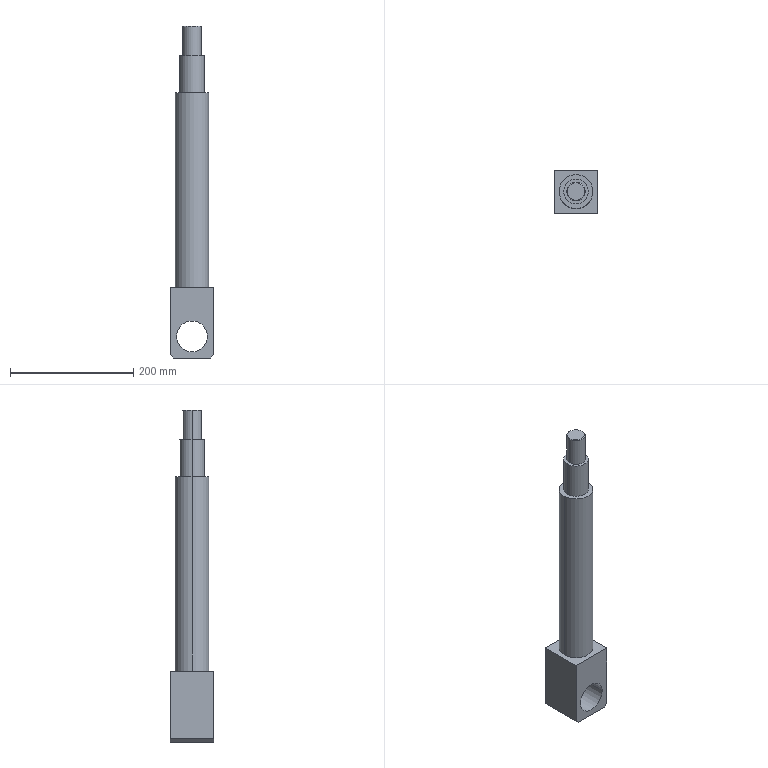Part | STEP file | LM-05-1239_default | 1 solid | 21 faces | box 70 x 70 x 538 mm | volume 1281973 mm3 | plane 11 | cylinder 8 | cone 2 | commonest cylinder face diameters 30 x2 40 x2 50 x2 55 x2
STEP:
#1=CARTESIAN_POINT('',(0.,0.,0.));
#2=DIRECTION('',(0.,0.,1.));
#3=DIRECTION('',(1.,0.,0.));
#4=AXIS2_PLACEMENT_3D('',#1,#2,#3);
#5=CARTESIAN_POINT('',(-25.,-35.,-80.));
#6=VERTEX_POINT('',#5);
#7=CARTESIAN_POINT('',(-25.,35.,-80.));
#8=VERTEX_POINT('',#7);
#9=CARTESIAN_POINT('',(-25.,-35.,-80.));
#10=DIRECTION('',(0.,1.,0.));
#11=VECTOR('',#10,1.);
#12=LINE('',#9,#11);
#13=CARTESIAN_POINT('',(0.,-35.,-80.));
#14=DIRECTION('',(0.,1.,0.));
#15=DIRECTION('',(-1.,0.,0.));
#16=AXIS2_PLACEMENT_3D('',#13,#14,#15);
#17=CYLINDRICAL_SURFACE('',#16,25.);
#18=CARTESIAN_POINT('',(6.283,0.));
#19=DIRECTION('',(0.,1.));
#20=VECTOR('',#19,1.);
#21=LINE('',#18,#20);
#22=(GEOMETRIC_REPRESENTATION_CONTEXT(2)PARAMETRIC_REPRESENTATION_CONTEXT()REPRESENTATION_CONTEXT('',''));
#23=DEFINITIONAL_REPRESENTATION('',(#21),#22);
#24=PCURVE('',#17,#23);
#25=CARTESIAN_POINT('',(0.,-35.,-80.));
#26=DIRECTION('',(0.,1.,0.));
#27=DIRECTION('',(-1.,0.,0.));
#28=AXIS2_PLACEMENT_3D('',#25,#26,#27);
#29=CYLINDRICAL_SURFACE('',#28,25.);
#30=CARTESIAN_POINT('',(0.,0.));
#31=DIRECTION('',(0.,1.));
#32=VECTOR('',#31,1.);
#33=LINE('',#30,#32);
#34=(GEOMETRIC_REPRESENTATION_CONTEXT(2)PARAMETRIC_REPRESENTATION_CONTEXT()REPRESENTATION_CONTEXT('',''));
#35=DEFINITIONAL_REPRESENTATION('',(#33),#34);
#36=PCURVE('',#29,#35);
#37=SURFACE_CURVE('',#12,(#24,#36),.PCURVE_S1.);
#38=EDGE_CURVE('',#6,#8,#37,.T.);
#39=ORIENTED_EDGE('',*,*,#38,.T.);
#40=CARTESIAN_POINT('',(25.,35.,-80.));
#41=VERTEX_POINT('',#40);
#42=CARTESIAN_POINT('',(0.,35.,-80.));
#43=DIRECTION('',(0.,1.,0.));
#44=DIRECTION('',(-1.,0.,0.));
#45=AXIS2_PLACEMENT_3D('',#42,#43,#44);
#46=CIRCLE('',#45,25.);
#47=CARTESIAN_POINT('',(0.,70.));
#48=DIRECTION('',(1.,0.));
#49=VECTOR('',#48,1.);
#50=LINE('',#47,#49);
#51=(GEOMETRIC_REPRESENTATION_CONTEXT(2)PARAMETRIC_REPRESENTATION_CONTEXT()REPRESENTATION_CONTEXT('',''));
#52=DEFINITIONAL_REPRESENTATION('',(#50),#51);
#53=PCURVE('',#17,#52);
#54=CARTESIAN_POINT('',(35.,35.,-115.));
#55=DIRECTION('',(0.,-1.,0.));
#56=DIRECTION('',(0.,0.,-1.));
#57=AXIS2_PLACEMENT_3D('',#54,#55,#56);
#58=PLANE('',#57);
#59=CARTESIAN_POINT('',(-35.,-60.));
#60=CARTESIAN_POINT('',(-78.301,-60.));
#61=CARTESIAN_POINT('',(-56.651,-22.5));
#62=CARTESIAN_POINT('',(-35.,15.));
#63=CARTESIAN_POINT('',(-13.349,-22.5));
#64=CARTESIAN_POINT('',(8.301,-60.));
#65=CARTESIAN_POINT('',(-35.,-60.));
#66=(BOUNDED_CURVE()B_SPLINE_CURVE(2,(#59,#60,#61,#62,#63,#64,#65),.UNSPECIFIED.,.T.,.F.)B_SPLINE_CURVE_WITH_KNOTS((1,2,2,2,2,1),(-2.094,0.,2.094,4.189,6.283,8.378),.UNSPECIFIED.)CURVE()GEOMETRIC_REPRESENTATION_ITEM()RATIONAL_B_SPLINE_CURVE((1.,0.5,1.,0.5,1.,0.5,1.))REPRESENTATION_ITEM(''));
#67=(GEOMETRIC_REPRESENTATION_CONTEXT(2)PARAMETRIC_REPRESENTATION_CONTEXT()REPRESENTATION_CONTEXT('',''));
#68=DEFINITIONAL_REPRESENTATION('',(#66),#67);
#69=PCURVE('',#58,#68);
#70=SURFACE_CURVE('',#46,(#53,#69),.PCURVE_S1.);
#71=EDGE_CURVE('',#41,#8,#70,.T.);
#72=ORIENTED_EDGE('',*,*,#71,.F.);
#73=CARTESIAN_POINT('',(25.,-35.,-80.));
#74=VERTEX_POINT('',#73);
#75=CARTESIAN_POINT('',(25.,-35.,-80.));
#76=DIRECTION('',(0.,1.,0.));
#77=VECTOR('',#76,1.);
#78=LINE('',#75,#77);
#79=CARTESIAN_POINT('',(3.142,0.));
#80=DIRECTION('',(0.,1.));
#81=VECTOR('',#80,1.);
#82=LINE('',#79,#81);
#83=(GEOMETRIC_REPRESENTATION_CONTEXT(2)PARAMETRIC_REPRESENTATION_CONTEXT()REPRESENTATION_CONTEXT('',''));
#84=DEFINITIONAL_REPRESENTATION('',(#82),#83);
#85=PCURVE('',#17,#84);
#86=CARTESIAN_POINT('',(3.142,0.));
#87=DIRECTION('',(0.,1.));
#88=VECTOR('',#87,1.);
#89=LINE('',#86,#88);
#90=(GEOMETRIC_REPRESENTATION_CONTEXT(2)PARAMETRIC_REPRESENTATION_CONTEXT()REPRESENTATION_CONTEXT('',''));
#91=DEFINITIONAL_REPRESENTATION('',(#89),#90);
#92=PCURVE('',#29,#91);
#93=SURFACE_CURVE('',#78,(#85,#92),.PCURVE_S1.);
#94=EDGE_CURVE('',#74,#41,#93,.T.);
#95=ORIENTED_EDGE('',*,*,#94,.F.);
#96=CARTESIAN_POINT('',(0.,-35.,-80.));
#97=DIRECTION('',(0.,1.,0.));
#98=DIRECTION('',(-1.,0.,0.));
#99=AXIS2_PLACEMENT_3D('',#96,#97,#98);
#100=CIRCLE('',#99,25.);
#101=CARTESIAN_POINT('',(0.,0.));
#102=DIRECTION('',(1.,0.));
#103=VECTOR('',#102,1.);
#104=LINE('',#101,#103);
#105=(GEOMETRIC_REPRESENTATION_CONTEXT(2)PARAMETRIC_REPRESENTATION_CONTEXT()REPRESENTATION_CONTEXT('',''));
#106=DEFINITIONAL_REPRESENTATION('',(#104),#105);
#107=PCURVE('',#17,#106);
#108=CARTESIAN_POINT('',(35.,-35.,-115.));
#109=DIRECTION('',(0.,1.,0.));
#110=DIRECTION('',(0.,0.,1.));
#111=AXIS2_PLACEMENT_3D('',#108,#109,#110);
#112=PLANE('',#111);
#113=CARTESIAN_POINT('',(35.,-35.));
#114=DIRECTION('',(0.,-1.));
#115=AXIS2_PLACEMENT_2D('',#113,#114);
#116=CIRCLE('',#115,25.);
#117=(GEOMETRIC_REPRESENTATION_CONTEXT(2)PARAMETRIC_REPRESENTATION_CONTEXT()REPRESENTATION_CONTEXT('',''));
#118=DEFINITIONAL_REPRESENTATION('',(#116),#117);
#119=PCURVE('',#112,#118);
#120=SURFACE_CURVE('',#100,(#107,#119),.PCURVE_S1.);
#121=EDGE_CURVE('',#74,#6,#120,.T.);
#122=ORIENTED_EDGE('',*,*,#121,.T.);
#123=EDGE_LOOP('',(#39,#72,#95,#122));
#124=FACE_BOUND('',#123,.F.);
#125=ADVANCED_FACE('',(#124),#17,.F.);
#126=CARTESIAN_POINT('',(20.,0.,315.));
#127=VERTEX_POINT('',#126);
#128=CARTESIAN_POINT('',(-20.,0.,315.));
#129=VERTEX_POINT('',#128);
#130=CARTESIAN_POINT('',(0.,0.,315.));
#131=DIRECTION('',(0.,0.,1.));
#132=DIRECTION('',(1.,0.,0.));
#133=AXIS2_PLACEMENT_3D('',#130,#131,#132);
#134=CIRCLE('',#133,20.);
#135=CARTESIAN_POINT('',(0.,0.,0.));
#136=DIRECTION('',(0.,0.,1.));
#137=DIRECTION('',(1.,0.,0.));
#138=AXIS2_PLACEMENT_3D('',#135,#136,#137);
#139=CYLINDRICAL_SURFACE('',#138,20.);
#140=CARTESIAN_POINT('',(0.,315.));
#141=DIRECTION('',(1.,0.));
#142=VECTOR('',#141,1.);
#143=LINE('',#140,#142);
#144=(GEOMETRIC_REPRESENTATION_CONTEXT(2)PARAMETRIC_REPRESENTATION_CONTEXT()REPRESENTATION_CONTEXT('',''));
#145=DEFINITIONAL_REPRESENTATION('',(#143),#144);
#146=PCURVE('',#139,#145);
#147=CARTESIAN_POINT('',(0.,20.,315.));
#148=DIRECTION('',(0.,0.,1.));
#149=DIRECTION('',(1.,0.,0.));
#150=AXIS2_PLACEMENT_3D('',#147,#148,#149);
#151=PLANE('',#150);
#152=CARTESIAN_POINT('',(0.,-20.));
#153=DIRECTION('',(1.,0.));
#154=AXIS2_PLACEMENT_2D('',#152,#153);
#155=CIRCLE('',#154,20.);
#156=(GEOMETRIC_REPRESENTATION_CONTEXT(2)PARAMETRIC_REPRESENTATION_CONTEXT()REPRESENTATION_CONTEXT('',''));
#157=DEFINITIONAL_REPRESENTATION('',(#155),#156);
#158=PCURVE('',#151,#157);
#159=SURFACE_CURVE('',#134,(#146,#158),.PCURVE_S1.);
#160=EDGE_CURVE('',#127,#129,#159,.T.);
#161=ORIENTED_EDGE('',*,*,#160,.T.);
#162=CARTESIAN_POINT('',(-20.,0.,375.));
#163=VERTEX_POINT('',#162);
#164=CARTESIAN_POINT('',(-20.,0.,0.));
#165=DIRECTION('',(0.,0.,1.));
#166=VECTOR('',#165,1.);
#167=LINE('',#164,#166);
#168=CARTESIAN_POINT('',(3.142,0.));
#169=DIRECTION('',(0.,1.));
#170=VECTOR('',#169,1.);
#171=LINE('',#168,#170);
#172=(GEOMETRIC_REPRESENTATION_CONTEXT(2)PARAMETRIC_REPRESENTATION_CONTEXT()REPRESENTATION_CONTEXT('',''));
#173=DEFINITIONAL_REPRESENTATION('',(#171),#172);
#174=PCURVE('',#139,#173);
#175=CARTESIAN_POINT('',(0.,0.,0.));
#176=DIRECTION('',(0.,0.,1.));
#177=DIRECTION('',(1.,0.,0.));
#178=AXIS2_PLACEMENT_3D('',#175,#176,#177);
#179=CYLINDRICAL_SURFACE('',#178,20.);
#180=CARTESIAN_POINT('',(3.142,0.));
#181=DIRECTION('',(0.,1.));
#182=VECTOR('',#181,1.);
#183=LINE('',#180,#182);
#184=(GEOMETRIC_REPRESENTATION_CONTEXT(2)PARAMETRIC_REPRESENTATION_CONTEXT()REPRESENTATION_CONTEXT('',''));
#185=DEFINITIONAL_REPRESENTATION('',(#183),#184);
#186=PCURVE('',#179,#185);
#187=SURFACE_CURVE('',#167,(#174,#186),.PCURVE_S1.);
#188=EDGE_CURVE('',#129,#163,#187,.T.);
#189=ORIENTED_EDGE('',*,*,#188,.T.);
#190=CARTESIAN_POINT('',(20.,0.,375.));
#191=VERTEX_POINT('',#190);
#192=CARTESIAN_POINT('',(0.,0.,375.));
#193=DIRECTION('',(0.,0.,1.));
#194=DIRECTION('',(1.,0.,0.));
#195=AXIS2_PLACEMENT_3D('',#192,#193,#194);
#196=CIRCLE('',#195,20.);
#197=CARTESIAN_POINT('',(0.,375.));
#198=DIRECTION('',(1.,0.));
#199=VECTOR('',#198,1.);
#200=LINE('',#197,#199);
#201=(GEOMETRIC_REPRESENTATION_CONTEXT(2)PARAMETRIC_REPRESENTATION_CONTEXT()REPRESENTATION_CONTEXT('',''));
#202=DEFINITIONAL_REPRESENTATION('',(#200),#201);
#203=PCURVE('',#139,#202);
#204=CARTESIAN_POINT('',(0.,0.,375.));
#205=DIRECTION('',(0.,0.,1.));
#206=DIRECTION('',(1.,0.,0.));
#207=AXIS2_PLACEMENT_3D('',#204,#205,#206);
#208=PLANE('',#207);
#209=CARTESIAN_POINT('',(0.,0.));
#210=DIRECTION('',(1.,0.));
#211=AXIS2_PLACEMENT_2D('',#209,#210);
#212=CIRCLE('',#211,20.);
#213=(GEOMETRIC_REPRESENTATION_CONTEXT(2)PARAMETRIC_REPRESENTATION_CONTEXT()REPRESENTATION_CONTEXT('',''));
#214=DEFINITIONAL_REPRESENTATION('',(#212),#213);
#215=PCURVE('',#208,#214);
#216=SURFACE_CURVE('',#196,(#203,#215),.PCURVE_S1.);
#217=EDGE_CURVE('',#191,#163,#216,.T.);
#218=ORIENTED_EDGE('',*,*,#217,.F.);
#219=CARTESIAN_POINT('',(20.,0.,0.));
#220=DIRECTION('',(0.,0.,1.));
#221=VECTOR('',#220,1.);
#222=LINE('',#219,#221);
#223=CARTESIAN_POINT('',(0.,0.));
#224=DIRECTION('',(0.,1.));
#225=VECTOR('',#224,1.);
#226=LINE('',#223,#225);
#227=(GEOMETRIC_REPRESENTATION_CONTEXT(2)PARAMETRIC_REPRESENTATION_CONTEXT()REPRESENTATION_CONTEXT('',''));
#228=DEFINITIONAL_REPRESENTATION('',(#226),#227);
#229=PCURVE('',#139,#228);
#230=CARTESIAN_POINT('',(6.283,0.));
#231=DIRECTION('',(0.,1.));
#232=VECTOR('',#231,1.);
#233=LINE('',#230,#232);
#234=(GEOMETRIC_REPRESENTATION_CONTEXT(2)PARAMETRIC_REPRESENTATION_CONTEXT()REPRESENTATION_CONTEXT('',''));
#235=DEFINITIONAL_REPRESENTATION('',(#233),#234);
#236=PCURVE('',#179,#235);
#237=SURFACE_CURVE('',#222,(#229,#236),.PCURVE_S1.);
#238=EDGE_CURVE('',#127,#191,#237,.T.);
#239=ORIENTED_EDGE('',*,*,#238,.F.);
#240=EDGE_LOOP('',(#161,#189,#218,#239));
#241=FACE_BOUND('',#240,.T.);
#242=ADVANCED_FACE('',(#241),#139,.T.);
#243=CARTESIAN_POINT('',(27.5,0.,0.));
#244=VERTEX_POINT('',#243);
#245=CARTESIAN_POINT('',(-27.5,0.,0.));
#246=VERTEX_POINT('',#245);
#247=CARTESIAN_POINT('',(0.,0.,0.));
#248=DIRECTION('',(0.,0.,1.));
#249=DIRECTION('',(1.,0.,0.));
#250=AXIS2_PLACEMENT_3D('',#247,#248,#249);
#251=CIRCLE('',#250,27.5);
#252=CARTESIAN_POINT('',(0.,0.,0.));
#253=DIRECTION('',(0.,0.,1.));
#254=DIRECTION('',(1.,0.,0.));
#255=AXIS2_PLACEMENT_3D('',#252,#253,#254);
#256=CYLINDRICAL_SURFACE('',#255,27.5);
#257=CARTESIAN_POINT('',(0.,0.));
#258=DIRECTION('',(1.,0.));
#259=VECTOR('',#258,1.);
#260=LINE('',#257,#259);
#261=(GEOMETRIC_REPRESENTATION_CONTEXT(2)PARAMETRIC_REPRESENTATION_CONTEXT()REPRESENTATION_CONTEXT('',''));
#262=DEFINITIONAL_REPRESENTATION('',(#260),#261);
#263=PCURVE('',#256,#262);
#264=CARTESIAN_POINT('',(0.,0.,0.));
#265=DIRECTION('',(0.,0.,-1.));
#266=DIRECTION('',(-1.,0.,0.));
#267=AXIS2_PLACEMENT_3D('',#264,#265,#266);
#268=PLANE('',#267);
#269=CARTESIAN_POINT('',(-27.5,0.));
#270=CARTESIAN_POINT('',(-27.5,47.631));
#271=CARTESIAN_POINT('',(13.75,23.816));
#272=CARTESIAN_POINT('',(55.,0.));
#273=CARTESIAN_POINT('',(13.75,-23.816));
#274=CARTESIAN_POINT('',(-27.5,-47.631));
#275=CARTESIAN_POINT('',(-27.5,0.));
#276=(BOUNDED_CURVE()B_SPLINE_CURVE(2,(#269,#270,#271,#272,#273,#274,#275),.UNSPECIFIED.,.T.,.F.)B_SPLINE_CURVE_WITH_KNOTS((1,2,2,2,2,1),(-2.094,0.,2.094,4.189,6.283,8.378),.UNSPECIFIED.)CURVE()GEOMETRIC_REPRESENTATION_ITEM()RATIONAL_B_SPLINE_CURVE((1.,0.5,1.,0.5,1.,0.5,1.))REPRESENTATION_ITEM(''));
#277=(GEOMETRIC_REPRESENTATION_CONTEXT(2)PARAMETRIC_REPRESENTATION_CONTEXT()REPRESENTATION_CONTEXT('',''));
#278=DEFINITIONAL_REPRESENTATION('',(#276),#277);
#279=PCURVE('',#268,#278);
#280=SURFACE_CURVE('',#251,(#263,#279),.PCURVE_S1.);
#281=EDGE_CURVE('',#244,#246,#280,.T.);
#282=ORIENTED_EDGE('',*,*,#281,.T.);
#283=CARTESIAN_POINT('',(-27.5,0.,315.));
#284=VERTEX_POINT('',#283);
#285=CARTESIAN_POINT('',(-27.5,0.,0.));
#286=DIRECTION('',(0.,0.,1.));
#287=VECTOR('',#286,1.);
#288=LINE('',#285,#287);
#289=CARTESIAN_POINT('',(3.142,0.));
#290=DIRECTION('',(0.,1.));
#291=VECTOR('',#290,1.);
#292=LINE('',#289,#291);
#293=(GEOMETRIC_REPRESENTATION_CONTEXT(2)PARAMETRIC_REPRESENTATION_CONTEXT()REPRESENTATION_CONTEXT('',''));
#294=DEFINITIONAL_REPRESENTATION('',(#292),#293);
#295=PCURVE('',#256,#294);
#296=CARTESIAN_POINT('',(0.,0.,0.));
#297=DIRECTION('',(0.,0.,1.));
#298=DIRECTION('',(1.,0.,0.));
#299=AXIS2_PLACEMENT_3D('',#296,#297,#298);
#300=CYLINDRICAL_SURFACE('',#299,27.5);
#301=CARTESIAN_POINT('',(3.142,0.));
#302=DIRECTION('',(0.,1.));
#303=VECTOR('',#302,1.);
#304=LINE('',#301,#303);
#305=(GEOMETRIC_REPRESENTATION_CONTEXT(2)PARAMETRIC_REPRESENTATION_CONTEXT()REPRESENTATION_CONTEXT('',''));
#306=DEFINITIONAL_REPRESENTATION('',(#304),#305);
#307=PCURVE('',#300,#306);
#308=SURFACE_CURVE('',#288,(#295,#307),.PCURVE_S1.);
#309=EDGE_CURVE('',#246,#284,#308,.T.);
#310=ORIENTED_EDGE('',*,*,#309,.T.);
#311=CARTESIAN_POINT('',(27.5,0.,315.));
#312=VERTEX_POINT('',#311);
#313=CARTESIAN_POINT('',(0.,0.,315.));
#314=DIRECTION('',(0.,0.,1.));
#315=DIRECTION('',(1.,0.,0.));
#316=AXIS2_PLACEMENT_3D('',#313,#314,#315);
#317=CIRCLE('',#316,27.5);
#318=CARTESIAN_POINT('',(0.,315.));
#319=DIRECTION('',(1.,0.));
#320=VECTOR('',#319,1.);
#321=LINE('',#318,#320);
#322=(GEOMETRIC_REPRESENTATION_CONTEXT(2)PARAMETRIC_REPRESENTATION_CONTEXT()REPRESENTATION_CONTEXT('',''));
#323=DEFINITIONAL_REPRESENTATION('',(#321),#322);
#324=PCURVE('',#256,#323);
#325=CARTESIAN_POINT('',(0.,-20.));
#326=DIRECTION('',(1.,0.));
#327=AXIS2_PLACEMENT_2D('',#325,#326);
#328=CIRCLE('',#327,27.5);
#329=(GEOMETRIC_REPRESENTATION_CONTEXT(2)PARAMETRIC_REPRESENTATION_CONTEXT()REPRESENTATION_CONTEXT('',''));
#330=DEFINITIONAL_REPRESENTATION('',(#328),#329);
#331=PCURVE('',#151,#330);
#332=SURFACE_CURVE('',#317,(#324,#331),.PCURVE_S1.);
#333=EDGE_CURVE('',#312,#284,#332,.T.);
#334=ORIENTED_EDGE('',*,*,#333,.F.);
#335=CARTESIAN_POINT('',(27.5,0.,0.));
#336=DIRECTION('',(0.,0.,1.));
#337=VECTOR('',#336,1.);
#338=LINE('',#335,#337);
#339=CARTESIAN_POINT('',(0.,0.));
#340=DIRECTION('',(0.,1.));
#341=VECTOR('',#340,1.);
#342=LINE('',#339,#341);
#343=(GEOMETRIC_REPRESENTATION_CONTEXT(2)PARAMETRIC_REPRESENTATION_CONTEXT()REPRESENTATION_CONTEXT('',''));
#344=DEFINITIONAL_REPRESENTATION('',(#342),#343);
#345=PCURVE('',#256,#344);
#346=CARTESIAN_POINT('',(6.283,0.));
#347=DIRECTION('',(0.,1.));
#348=VECTOR('',#347,1.);
#349=LINE('',#346,#348);
#350=(GEOMETRIC_REPRESENTATION_CONTEXT(2)PARAMETRIC_REPRESENTATION_CONTEXT()REPRESENTATION_CONTEXT('',''));
#351=DEFINITIONAL_REPRESENTATION('',(#349),#350);
#352=PCURVE('',#300,#351);
#353=SURFACE_CURVE('',#338,(#345,#352),.PCURVE_S1.);
#354=EDGE_CURVE('',#244,#312,#353,.T.);
#355=ORIENTED_EDGE('',*,*,#354,.F.);
#356=EDGE_LOOP('',(#282,#310,#334,#355));
#357=FACE_BOUND('',#356,.T.);
#358=ADVANCED_FACE('',(#357),#256,.T.);
#359=CARTESIAN_POINT('',(15.,0.,375.));
#360=VERTEX_POINT('',#359);
#361=CARTESIAN_POINT('',(-15.,0.,375.));
#362=VERTEX_POINT('',#361);
#363=CARTESIAN_POINT('',(0.,0.,375.));
#364=DIRECTION('',(0.,0.,1.));
#365=DIRECTION('',(1.,0.,0.));
#366=AXIS2_PLACEMENT_3D('',#363,#364,#365);
#367=CIRCLE('',#366,15.);
#368=CARTESIAN_POINT('',(0.,0.,0.));
#369=DIRECTION('',(0.,0.,1.));
#370=DIRECTION('',(1.,0.,0.));
#371=AXIS2_PLACEMENT_3D('',#368,#369,#370);
#372=CYLINDRICAL_SURFACE('',#371,15.);
#373=CARTESIAN_POINT('',(0.,375.));
#374=DIRECTION('',(1.,0.));
#375=VECTOR('',#374,1.);
#376=LINE('',#373,#375);
#377=(GEOMETRIC_REPRESENTATION_CONTEXT(2)PARAMETRIC_REPRESENTATION_CONTEXT()REPRESENTATION_CONTEXT('',''));
#378=DEFINITIONAL_REPRESENTATION('',(#376),#377);
#379=PCURVE('',#372,#378);
#380=CARTESIAN_POINT('',(0.,0.));
#381=DIRECTION('',(1.,0.));
#382=AXIS2_PLACEMENT_2D('',#380,#381);
#383=CIRCLE('',#382,15.);
#384=(GEOMETRIC_REPRESENTATION_CONTEXT(2)PARAMETRIC_REPRESENTATION_CONTEXT()REPRESENTATION_CONTEXT('',''));
#385=DEFINITIONAL_REPRESENTATION('',(#383),#384);
#386=PCURVE('',#208,#385);
#387=SURFACE_CURVE('',#367,(#379,#386),.PCURVE_S1.);
#388=EDGE_CURVE('',#360,#362,#387,.T.);
#389=ORIENTED_EDGE('',*,*,#388,.T.);
#390=CARTESIAN_POINT('',(-15.,0.,422.));
#391=VERTEX_POINT('',#390);
#392=CARTESIAN_POINT('',(-15.,0.,0.));
#393=DIRECTION('',(0.,0.,1.));
#394=VECTOR('',#393,1.);
#395=LINE('',#392,#394);
#396=CARTESIAN_POINT('',(3.142,0.));
#397=DIRECTION('',(0.,1.));
#398=VECTOR('',#397,1.);
#399=LINE('',#396,#398);
#400=(GEOMETRIC_REPRESENTATION_CONTEXT(2)PARAMETRIC_REPRESENTATION_CONTEXT()REPRESENTATION_CONTEXT('',''));
#401=DEFINITIONAL_REPRESENTATION('',(#399),#400);
#402=PCURVE('',#372,#401);
#403=CARTESIAN_POINT('',(0.,0.,0.));
#404=DIRECTION('',(0.,0.,1.));
#405=DIRECTION('',(1.,0.,0.));
#406=AXIS2_PLACEMENT_3D('',#403,#404,#405);
#407=CYLINDRICAL_SURFACE('',#406,15.);
#408=CARTESIAN_POINT('',(3.142,0.));
#409=DIRECTION('',(0.,1.));
#410=VECTOR('',#409,1.);
#411=LINE('',#408,#410);
#412=(GEOMETRIC_REPRESENTATION_CONTEXT(2)PARAMETRIC_REPRESENTATION_CONTEXT()REPRESENTATION_CONTEXT('',''));
#413=DEFINITIONAL_REPRESENTATION('',(#411),#412);
#414=PCURVE('',#407,#413);
#415=SURFACE_CURVE('',#395,(#402,#414),.PCURVE_S1.);
#416=EDGE_CURVE('',#362,#391,#415,.T.);
#417=ORIENTED_EDGE('',*,*,#416,.T.);
#418=CARTESIAN_POINT('',(15.,0.,422.));
#419=VERTEX_POINT('',#418);
#420=CARTESIAN_POINT('',(0.,0.,422.));
#421=DIRECTION('',(0.,0.,1.));
#422=DIRECTION('',(1.,0.,0.));
#423=AXIS2_PLACEMENT_3D('',#420,#421,#422);
#424=CIRCLE('',#423,15.);
#425=CARTESIAN_POINT('',(0.,422.));
#426=DIRECTION('',(1.,0.));
#427=VECTOR('',#426,1.);
#428=LINE('',#425,#427);
#429=(GEOMETRIC_REPRESENTATION_CONTEXT(2)PARAMETRIC_REPRESENTATION_CONTEXT()REPRESENTATION_CONTEXT('',''));
#430=DEFINITIONAL_REPRESENTATION('',(#428),#429);
#431=PCURVE('',#372,#430);
#432=CARTESIAN_POINT('',(0.,0.,422.));
#433=DIRECTION('',(0.,0.,-1.));
#434=DIRECTION('',(-1.,0.,0.));
#435=AXIS2_PLACEMENT_3D('',#432,#433,#434);
#436=CONICAL_SURFACE('',#435,15.,0.7854);
#437=CARTESIAN_POINT('',(3.142,0.));
#438=DIRECTION('',(-1.,0.));
#439=VECTOR('',#438,1.);
#440=LINE('',#437,#439);
#441=(GEOMETRIC_REPRESENTATION_CONTEXT(2)PARAMETRIC_REPRESENTATION_CONTEXT()REPRESENTATION_CONTEXT('',''));
#442=DEFINITIONAL_REPRESENTATION('',(#440),#441);
#443=PCURVE('',#436,#442);
#444=SURFACE_CURVE('',#424,(#431,#443),.PCURVE_S1.);
#445=EDGE_CURVE('',#419,#391,#444,.T.);
#446=ORIENTED_EDGE('',*,*,#445,.F.);
#447=CARTESIAN_POINT('',(15.,0.,0.));
#448=DIRECTION('',(0.,0.,1.));
#449=VECTOR('',#448,1.);
#450=LINE('',#447,#449);
#451=CARTESIAN_POINT('',(0.,0.));
#452=DIRECTION('',(0.,1.));
#453=VECTOR('',#452,1.);
#454=LINE('',#451,#453);
#455=(GEOMETRIC_REPRESENTATION_CONTEXT(2)PARAMETRIC_REPRESENTATION_CONTEXT()REPRESENTATION_CONTEXT('',''));
#456=DEFINITIONAL_REPRESENTATION('',(#454),#455);
#457=PCURVE('',#372,#456);
#458=CARTESIAN_POINT('',(6.283,0.));
#459=DIRECTION('',(0.,1.));
#460=VECTOR('',#459,1.);
#461=LINE('',#458,#460);
#462=(GEOMETRIC_REPRESENTATION_CONTEXT(2)PARAMETRIC_REPRESENTATION_CONTEXT()REPRESENTATION_CONTEXT('',''));
#463=DEFINITIONAL_REPRESENTATION('',(#461),#462);
#464=PCURVE('',#407,#463);
#465=SURFACE_CURVE('',#450,(#457,#464),.PCURVE_S1.);
#466=EDGE_CURVE('',#360,#419,#465,.T.);
#467=ORIENTED_EDGE('',*,*,#466,.F.);
#468=EDGE_LOOP('',(#389,#417,#446,#467));
#469=FACE_BOUND('',#468,.T.);
#470=ADVANCED_FACE('',(#469),#372,.T.);
#471=CARTESIAN_POINT('',(14.,0.,423.));
#472=VERTEX_POINT('',#471);
#473=CARTESIAN_POINT('',(-14.,0.,423.));
#474=VERTEX_POINT('',#473);
#475=CARTESIAN_POINT('',(0.,0.,423.));
#476=DIRECTION('',(0.,0.,1.));
#477=DIRECTION('',(1.,0.,0.));
#478=AXIS2_PLACEMENT_3D('',#475,#476,#477);
#479=CIRCLE('',#478,14.);
#480=CARTESIAN_POINT('',(3.142,-1.));
#481=DIRECTION('',(-1.,0.));
#482=VECTOR('',#481,1.);
#483=LINE('',#480,#482);
#484=(GEOMETRIC_REPRESENTATION_CONTEXT(2)PARAMETRIC_REPRESENTATION_CONTEXT()REPRESENTATION_CONTEXT('',''));
#485=DEFINITIONAL_REPRESENTATION('',(#483),#484);
#486=PCURVE('',#436,#485);
#487=CARTESIAN_POINT('',(0.,0.,423.));
#488=DIRECTION('',(0.,0.,-1.));
#489=DIRECTION('',(-1.,0.,0.));
#490=AXIS2_PLACEMENT_3D('',#487,#488,#489);
#491=PLANE('',#490);
#492=CARTESIAN_POINT('',(-14.,0.));
#493=CARTESIAN_POINT('',(-14.,24.249));
#494=CARTESIAN_POINT('',(7.,12.124));
#495=CARTESIAN_POINT('',(28.,0.));
#496=CARTESIAN_POINT('',(7.,-12.124));
#497=CARTESIAN_POINT('',(-14.,-24.249));
#498=CARTESIAN_POINT('',(-14.,0.));
#499=(BOUNDED_CURVE()B_SPLINE_CURVE(2,(#492,#493,#494,#495,#496,#497,#498),.UNSPECIFIED.,.T.,.F.)B_SPLINE_CURVE_WITH_KNOTS((1,2,2,2,2,1),(-2.094,0.,2.094,4.189,6.283,8.378),.UNSPECIFIED.)CURVE()GEOMETRIC_REPRESENTATION_ITEM()RATIONAL_B_SPLINE_CURVE((1.,0.5,1.,0.5,1.,0.5,1.))REPRESENTATION_ITEM(''));
#500=(GEOMETRIC_REPRESENTATION_CONTEXT(2)PARAMETRIC_REPRESENTATION_CONTEXT()REPRESENTATION_CONTEXT('',''));
#501=DEFINITIONAL_REPRESENTATION('',(#499),#500);
#502=PCURVE('',#491,#501);
#503=SURFACE_CURVE('',#479,(#486,#502),.PCURVE_S1.);
#504=EDGE_CURVE('',#472,#474,#503,.T.);
#505=ORIENTED_EDGE('',*,*,#504,.F.);
#506=CARTESIAN_POINT('',(15.,0.,422.));
#507=DIRECTION('',(0.7071,0.,-0.7071));
#508=VECTOR('',#507,1.);
#509=LINE('',#506,#508);
#510=CARTESIAN_POINT('',(3.142,0.));
#511=DIRECTION('',(0.,1.));
#512=VECTOR('',#511,1.);
#513=LINE('',#510,#512);
#514=(GEOMETRIC_REPRESENTATION_CONTEXT(2)PARAMETRIC_REPRESENTATION_CONTEXT()REPRESENTATION_CONTEXT('',''));
#515=DEFINITIONAL_REPRESENTATION('',(#513),#514);
#516=PCURVE('',#436,#515);
#517=CARTESIAN_POINT('',(0.,0.,422.));
#518=DIRECTION('',(0.,0.,-1.));
#519=DIRECTION('',(-1.,0.,0.));
#520=AXIS2_PLACEMENT_3D('',#517,#518,#519);
#521=CONICAL_SURFACE('',#520,15.,0.7854);
#522=CARTESIAN_POINT('',(3.142,0.));
#523=DIRECTION('',(0.,1.));
#524=VECTOR('',#523,1.);
#525=LINE('',#522,#524);
#526=(GEOMETRIC_REPRESENTATION_CONTEXT(2)PARAMETRIC_REPRESENTATION_CONTEXT()REPRESENTATION_CONTEXT('',''));
#527=DEFINITIONAL_REPRESENTATION('',(#525),#526);
#528=PCURVE('',#521,#527);
#529=SURFACE_CURVE('',#509,(#516,#528),.PCURVE_S1.);
#530=EDGE_CURVE('',#472,#419,#529,.T.);
#531=ORIENTED_EDGE('',*,*,#530,.T.);
#532=ORIENTED_EDGE('',*,*,#445,.T.);
#533=CARTESIAN_POINT('',(-15.,0.,422.));
#534=DIRECTION('',(-0.7071,0.,-0.7071));
#535=VECTOR('',#534,1.);
#536=LINE('',#533,#535);
#537=CARTESIAN_POINT('',(0.,0.));
#538=DIRECTION('',(0.,1.));
#539=VECTOR('',#538,1.);
#540=LINE('',#537,#539);
#541=(GEOMETRIC_REPRESENTATION_CONTEXT(2)PARAMETRIC_REPRESENTATION_CONTEXT()REPRESENTATION_CONTEXT('',''));
#542=DEFINITIONAL_REPRESENTATION('',(#540),#541);
#543=PCURVE('',#436,#542);
#544=CARTESIAN_POINT('',(6.283,0.));
#545=DIRECTION('',(0.,1.));
#546=VECTOR('',#545,1.);
#547=LINE('',#544,#546);
#548=(GEOMETRIC_REPRESENTATION_CONTEXT(2)PARAMETRIC_REPRESENTATION_CONTEXT()REPRESENTATION_CONTEXT('',''));
#549=DEFINITIONAL_REPRESENTATION('',(#547),#548);
#550=PCURVE('',#521,#549);
#551=SURFACE_CURVE('',#536,(#543,#550),.PCURVE_S1.);
#552=EDGE_CURVE('',#474,#391,#551,.T.);
#553=ORIENTED_EDGE('',*,*,#552,.F.);
#554=EDGE_LOOP('',(#505,#531,#532,#553));
#555=FACE_BOUND('',#554,.T.);
#556=ADVANCED_FACE('',(#555),#436,.T.);
#557=CARTESIAN_POINT('',(0.,0.,423.));
#558=DIRECTION('',(0.,0.,1.));
#559=DIRECTION('',(1.,0.,0.));
#560=AXIS2_PLACEMENT_3D('',#557,#558,#559);
#561=CIRCLE('',#560,14.);
#562=CARTESIAN_POINT('',(-14.,0.));
#563=CARTESIAN_POINT('',(-14.,24.249));
#564=CARTESIAN_POINT('',(7.,12.124));
#565=CARTESIAN_POINT('',(28.,0.));
#566=CARTESIAN_POINT('',(7.,-12.124));
#567=CARTESIAN_POINT('',(-14.,-24.249));
#568=CARTESIAN_POINT('',(-14.,0.));
#569=(BOUNDED_CURVE()B_SPLINE_CURVE(2,(#562,#563,#564,#565,#566,#567,#568),.UNSPECIFIED.,.T.,.F.)B_SPLINE_CURVE_WITH_KNOTS((1,2,2,2,2,1),(-2.094,0.,2.094,4.189,6.283,8.378),.UNSPECIFIED.)CURVE()GEOMETRIC_REPRESENTATION_ITEM()RATIONAL_B_SPLINE_CURVE((1.,0.5,1.,0.5,1.,0.5,1.))REPRESENTATION_ITEM(''));
#570=(GEOMETRIC_REPRESENTATION_CONTEXT(2)PARAMETRIC_REPRESENTATION_CONTEXT()REPRESENTATION_CONTEXT('',''));
#571=DEFINITIONAL_REPRESENTATION('',(#569),#570);
#572=PCURVE('',#491,#571);
#573=CARTESIAN_POINT('',(9.425,-1.));
#574=DIRECTION('',(-1.,0.));
#575=VECTOR('',#574,1.);
#576=LINE('',#573,#575);
#577=(GEOMETRIC_REPRESENTATION_CONTEXT(2)PARAMETRIC_REPRESENTATION_CONTEXT()REPRESENTATION_CONTEXT('',''));
#578=DEFINITIONAL_REPRESENTATION('',(#576),#577);
#579=PCURVE('',#521,#578);
#580=SURFACE_CURVE('',#561,(#572,#579),.PCURVE_S1.);
#581=EDGE_CURVE('',#474,#472,#580,.T.);
#582=ORIENTED_EDGE('',*,*,#581,.T.);
#583=ORIENTED_EDGE('',*,*,#504,.T.);
#584=EDGE_LOOP('',(#582,#583));
#585=FACE_BOUND('',#584,.T.);
#586=ADVANCED_FACE('',(#585),#491,.F.);
#587=ORIENTED_EDGE('',*,*,#530,.F.);
#588=ORIENTED_EDGE('',*,*,#581,.F.);
#589=ORIENTED_EDGE('',*,*,#552,.T.);
#590=CARTESIAN_POINT('',(0.,0.,422.));
#591=DIRECTION('',(0.,0.,1.));
#592=DIRECTION('',(1.,0.,0.));
#593=AXIS2_PLACEMENT_3D('',#590,#591,#592);
#594=CIRCLE('',#593,15.);
#595=CARTESIAN_POINT('',(9.425,0.));
#596=DIRECTION('',(-1.,0.));
#597=VECTOR('',#596,1.);
#598=LINE('',#595,#597);
#599=(GEOMETRIC_REPRESENTATION_CONTEXT(2)PARAMETRIC_REPRESENTATION_CONTEXT()REPRESENTATION_CONTEXT('',''));
#600=DEFINITIONAL_REPRESENTATION('',(#598),#599);
#601=PCURVE('',#521,#600);
#602=CARTESIAN_POINT('',(0.,422.));
#603=DIRECTION('',(1.,0.));
#604=VECTOR('',#603,1.);
#605=LINE('',#602,#604);
#606=(GEOMETRIC_REPRESENTATION_CONTEXT(2)PARAMETRIC_REPRESENTATION_CONTEXT()REPRESENTATION_CONTEXT('',''));
#607=DEFINITIONAL_REPRESENTATION('',(#605),#606);
#608=PCURVE('',#407,#607);
#609=SURFACE_CURVE('',#594,(#601,#608),.PCURVE_S1.);
#610=EDGE_CURVE('',#391,#419,#609,.T.);
#611=ORIENTED_EDGE('',*,*,#610,.T.);
#612=EDGE_LOOP('',(#587,#588,#589,#611));
#613=FACE_BOUND('',#612,.T.);
#614=ADVANCED_FACE('',(#613),#521,.T.);
#615=ORIENTED_EDGE('',*,*,#416,.F.);
#616=CARTESIAN_POINT('',(0.,0.,375.));
#617=DIRECTION('',(0.,0.,1.));
#618=DIRECTION('',(1.,0.,0.));
#619=AXIS2_PLACEMENT_3D('',#616,#617,#618);
#620=CIRCLE('',#619,15.);
#621=CARTESIAN_POINT('',(0.,375.));
#622=DIRECTION('',(1.,0.));
#623=VECTOR('',#622,1.);
#624=LINE('',#621,#623);
#625=(GEOMETRIC_REPRESENTATION_CONTEXT(2)PARAMETRIC_REPRESENTATION_CONTEXT()REPRESENTATION_CONTEXT('',''));
#626=DEFINITIONAL_REPRESENTATION('',(#624),#625);
#627=PCURVE('',#407,#626);
#628=CARTESIAN_POINT('',(0.,0.));
#629=DIRECTION('',(1.,0.));
#630=AXIS2_PLACEMENT_2D('',#628,#629);
#631=CIRCLE('',#630,15.);
#632=(GEOMETRIC_REPRESENTATION_CONTEXT(2)PARAMETRIC_REPRESENTATION_CONTEXT()REPRESENTATION_CONTEXT('',''));
#633=DEFINITIONAL_REPRESENTATION('',(#631),#632);
#634=PCURVE('',#208,#633);
#635=SURFACE_CURVE('',#620,(#627,#634),.PCURVE_S1.);
#636=EDGE_CURVE('',#362,#360,#635,.T.);
#637=ORIENTED_EDGE('',*,*,#636,.T.);
#638=ORIENTED_EDGE('',*,*,#466,.T.);
#639=ORIENTED_EDGE('',*,*,#610,.F.);
#640=EDGE_LOOP('',(#615,#637,#638,#639));
#641=FACE_BOUND('',#640,.T.);
#642=ADVANCED_FACE('',(#641),#407,.T.);
#643=ORIENTED_EDGE('',*,*,#388,.F.);
#644=ORIENTED_EDGE('',*,*,#636,.F.);
#645=EDGE_LOOP('',(#643,#644));
#646=FACE_BOUND('',#645,.T.);
#647=ORIENTED_EDGE('',*,*,#217,.T.);
#648=CARTESIAN_POINT('',(0.,0.,375.));
#649=DIRECTION('',(0.,0.,1.));
#650=DIRECTION('',(1.,0.,0.));
#651=AXIS2_PLACEMENT_3D('',#648,#649,#650);
#652=CIRCLE('',#651,20.);
#653=CARTESIAN_POINT('',(0.,0.));
#654=DIRECTION('',(1.,0.));
#655=AXIS2_PLACEMENT_2D('',#653,#654);
#656=CIRCLE('',#655,20.);
#657=(GEOMETRIC_REPRESENTATION_CONTEXT(2)PARAMETRIC_REPRESENTATION_CONTEXT()REPRESENTATION_CONTEXT('',''));
#658=DEFINITIONAL_REPRESENTATION('',(#656),#657);
#659=PCURVE('',#208,#658);
#660=CARTESIAN_POINT('',(0.,375.));
#661=DIRECTION('',(1.,0.));
#662=VECTOR('',#661,1.);
#663=LINE('',#660,#662);
#664=(GEOMETRIC_REPRESENTATION_CONTEXT(2)PARAMETRIC_REPRESENTATION_CONTEXT()REPRESENTATION_CONTEXT('',''));
#665=DEFINITIONAL_REPRESENTATION('',(#663),#664);
#666=PCURVE('',#179,#665);
#667=SURFACE_CURVE('',#652,(#659,#666),.PCURVE_S1.);
#668=EDGE_CURVE('',#163,#191,#667,.T.);
#669=ORIENTED_EDGE('',*,*,#668,.T.);
#670=EDGE_LOOP('',(#647,#669));
#671=FACE_BOUND('',#670,.T.);
#672=ADVANCED_FACE('',(#646,#671),#208,.T.);
#673=ORIENTED_EDGE('',*,*,#188,.F.);
#674=CARTESIAN_POINT('',(0.,0.,315.));
#675=DIRECTION('',(0.,0.,1.));
#676=DIRECTION('',(1.,0.,0.));
#677=AXIS2_PLACEMENT_3D('',#674,#675,#676);
#678=CIRCLE('',#677,20.);
#679=CARTESIAN_POINT('',(0.,315.));
#680=DIRECTION('',(1.,0.));
#681=VECTOR('',#680,1.);
#682=LINE('',#679,#681);
#683=(GEOMETRIC_REPRESENTATION_CONTEXT(2)PARAMETRIC_REPRESENTATION_CONTEXT()REPRESENTATION_CONTEXT('',''));
#684=DEFINITIONAL_REPRESENTATION('',(#682),#683);
#685=PCURVE('',#179,#684);
#686=CARTESIAN_POINT('',(0.,-20.));
#687=DIRECTION('',(1.,0.));
#688=AXIS2_PLACEMENT_2D('',#686,#687);
#689=CIRCLE('',#688,20.);
#690=(GEOMETRIC_REPRESENTATION_CONTEXT(2)PARAMETRIC_REPRESENTATION_CONTEXT()REPRESENTATION_CONTEXT('',''));
#691=DEFINITIONAL_REPRESENTATION('',(#689),#690);
#692=PCURVE('',#151,#691);
#693=SURFACE_CURVE('',#678,(#685,#692),.PCURVE_S1.);
#694=EDGE_CURVE('',#129,#127,#693,.T.);
#695=ORIENTED_EDGE('',*,*,#694,.T.);
#696=ORIENTED_EDGE('',*,*,#238,.T.);
#697=ORIENTED_EDGE('',*,*,#668,.F.);
#698=EDGE_LOOP('',(#673,#695,#696,#697));
#699=FACE_BOUND('',#698,.T.);
#700=ADVANCED_FACE('',(#699),#179,.T.);
#701=ORIENTED_EDGE('',*,*,#333,.T.);
#702=CARTESIAN_POINT('',(0.,0.,315.));
#703=DIRECTION('',(0.,0.,1.));
#704=DIRECTION('',(1.,0.,0.));
#705=AXIS2_PLACEMENT_3D('',#702,#703,#704);
#706=CIRCLE('',#705,27.5);
#707=CARTESIAN_POINT('',(0.,-20.));
#708=DIRECTION('',(1.,0.));
#709=AXIS2_PLACEMENT_2D('',#707,#708);
#710=CIRCLE('',#709,27.5);
#711=(GEOMETRIC_REPRESENTATION_CONTEXT(2)PARAMETRIC_REPRESENTATION_CONTEXT()REPRESENTATION_CONTEXT('',''));
#712=DEFINITIONAL_REPRESENTATION('',(#710),#711);
#713=PCURVE('',#151,#712);
#714=CARTESIAN_POINT('',(0.,315.));
#715=DIRECTION('',(1.,0.));
#716=VECTOR('',#715,1.);
#717=LINE('',#714,#716);
#718=(GEOMETRIC_REPRESENTATION_CONTEXT(2)PARAMETRIC_REPRESENTATION_CONTEXT()REPRESENTATION_CONTEXT('',''));
#719=DEFINITIONAL_REPRESENTATION('',(#717),#718);
#720=PCURVE('',#300,#719);
#721=SURFACE_CURVE('',#706,(#713,#720),.PCURVE_S1.);
#722=EDGE_CURVE('',#284,#312,#721,.T.);
#723=ORIENTED_EDGE('',*,*,#722,.T.);
#724=EDGE_LOOP('',(#701,#723));
#725=FACE_BOUND('',#724,.T.);
#726=ORIENTED_EDGE('',*,*,#160,.F.);
#727=ORIENTED_EDGE('',*,*,#694,.F.);
#728=EDGE_LOOP('',(#726,#727));
#729=FACE_BOUND('',#728,.T.);
#730=ADVANCED_FACE('',(#725,#729),#151,.T.);
#731=ORIENTED_EDGE('',*,*,#309,.F.);
#732=CARTESIAN_POINT('',(0.,0.,0.));
#733=DIRECTION('',(0.,0.,1.));
#734=DIRECTION('',(1.,0.,0.));
#735=AXIS2_PLACEMENT_3D('',#732,#733,#734);
#736=CIRCLE('',#735,27.5);
#737=CARTESIAN_POINT('',(0.,0.));
#738=DIRECTION('',(1.,0.));
#739=VECTOR('',#738,1.);
#740=LINE('',#737,#739);
#741=(GEOMETRIC_REPRESENTATION_CONTEXT(2)PARAMETRIC_REPRESENTATION_CONTEXT()REPRESENTATION_CONTEXT('',''));
#742=DEFINITIONAL_REPRESENTATION('',(#740),#741);
#743=PCURVE('',#300,#742);
#744=CARTESIAN_POINT('',(-27.5,0.));
#745=CARTESIAN_POINT('',(-27.5,47.631));
#746=CARTESIAN_POINT('',(13.75,23.816));
#747=CARTESIAN_POINT('',(55.,0.));
#748=CARTESIAN_POINT('',(13.75,-23.816));
#749=CARTESIAN_POINT('',(-27.5,-47.631));
#750=CARTESIAN_POINT('',(-27.5,0.));
#751=(BOUNDED_CURVE()B_SPLINE_CURVE(2,(#744,#745,#746,#747,#748,#749,#750),.UNSPECIFIED.,.T.,.F.)B_SPLINE_CURVE_WITH_KNOTS((1,2,2,2,2,1),(-2.094,0.,2.094,4.189,6.283,8.378),.UNSPECIFIED.)CURVE()GEOMETRIC_REPRESENTATION_ITEM()RATIONAL_B_SPLINE_CURVE((1.,0.5,1.,0.5,1.,0.5,1.))REPRESENTATION_ITEM(''));
#752=(GEOMETRIC_REPRESENTATION_CONTEXT(2)PARAMETRIC_REPRESENTATION_CONTEXT()REPRESENTATION_CONTEXT('',''));
#753=DEFINITIONAL_REPRESENTATION('',(#751),#752);
#754=PCURVE('',#268,#753);
#755=SURFACE_CURVE('',#736,(#743,#754),.PCURVE_S1.);
#756=EDGE_CURVE('',#246,#244,#755,.T.);
#757=ORIENTED_EDGE('',*,*,#756,.T.);
#758=ORIENTED_EDGE('',*,*,#354,.T.);
#759=ORIENTED_EDGE('',*,*,#722,.F.);
#760=EDGE_LOOP('',(#731,#757,#758,#759));
#761=FACE_BOUND('',#760,.T.);
#762=ADVANCED_FACE('',(#761),#300,.T.);
#763=CARTESIAN_POINT('',(-35.,35.,-110.));
#764=VERTEX_POINT('',#763);
#765=CARTESIAN_POINT('',(-35.,35.,0.));
#766=VERTEX_POINT('',#765);
#767=CARTESIAN_POINT('',(-35.,35.,-115.));
#768=DIRECTION('',(0.,0.,1.));
#769=VECTOR('',#768,1.);
#770=LINE('',#767,#769);
#771=CARTESIAN_POINT('',(-35.,35.,-115.));
#772=DIRECTION('',(1.,0.,0.));
#773=DIRECTION('',(0.,0.,-1.));
#774=AXIS2_PLACEMENT_3D('',#771,#772,#773);
#775=PLANE('',#774);
#776=CARTESIAN_POINT('',(0.,0.));
#777=DIRECTION('',(-1.,0.));
#778=VECTOR('',#777,1.);
#779=LINE('',#776,#778);
#780=(GEOMETRIC_REPRESENTATION_CONTEXT(2)PARAMETRIC_REPRESENTATION_CONTEXT()REPRESENTATION_CONTEXT('',''));
#781=DEFINITIONAL_REPRESENTATION('',(#779),#780);
#782=PCURVE('',#775,#781);
#783=CARTESIAN_POINT('',(0.,-70.));
#784=DIRECTION('',(-1.,0.));
#785=VECTOR('',#784,1.);
#786=LINE('',#783,#785);
#787=(GEOMETRIC_REPRESENTATION_CONTEXT(2)PARAMETRIC_REPRESENTATION_CONTEXT()REPRESENTATION_CONTEXT('',''));
#788=DEFINITIONAL_REPRESENTATION('',(#786),#787);
#789=PCURVE('',#58,#788);
#790=SURFACE_CURVE('',#770,(#782,#789),.PCURVE_S1.);
#791=EDGE_CURVE('',#764,#766,#790,.T.);
#792=ORIENTED_EDGE('',*,*,#791,.F.);
#793=CARTESIAN_POINT('',(-35.,-35.,-110.));
#794=VERTEX_POINT('',#793);
#795=CARTESIAN_POINT('',(-35.,-35.,-110.));
#796=DIRECTION('',(0.,-1.,0.));
#797=VECTOR('',#796,1.);
#798=LINE('',#795,#797);
#799=CARTESIAN_POINT('',(-5.,-70.));
#800=DIRECTION('',(0.,-1.));
#801=VECTOR('',#800,1.);
#802=LINE('',#799,#801);
#803=(GEOMETRIC_REPRESENTATION_CONTEXT(2)PARAMETRIC_REPRESENTATION_CONTEXT()REPRESENTATION_CONTEXT('',''));
#804=DEFINITIONAL_REPRESENTATION('',(#802),#803);
#805=PCURVE('',#775,#804);
#806=CARTESIAN_POINT('',(-30.,0.,-115.));
#807=DIRECTION('',(-0.7071,0.,-0.7071));
#808=DIRECTION('',(0.,-1.,0.));
#809=AXIS2_PLACEMENT_3D('',#806,#807,#808);
#810=PLANE('',#809);
#811=CARTESIAN_POINT('',(35.,7.071));
#812=DIRECTION('',(1.,0.));
#813=VECTOR('',#812,1.);
#814=LINE('',#811,#813);
#815=(GEOMETRIC_REPRESENTATION_CONTEXT(2)PARAMETRIC_REPRESENTATION_CONTEXT()REPRESENTATION_CONTEXT('',''));
#816=DEFINITIONAL_REPRESENTATION('',(#814),#815);
#817=PCURVE('',#810,#816);
#818=SURFACE_CURVE('',#798,(#805,#817),.PCURVE_S1.);
#819=EDGE_CURVE('',#764,#794,#818,.T.);
#820=ORIENTED_EDGE('',*,*,#819,.T.);
#821=CARTESIAN_POINT('',(-35.,-35.,0.));
#822=VERTEX_POINT('',#821);
#823=CARTESIAN_POINT('',(-35.,-35.,-115.));
#824=DIRECTION('',(0.,0.,1.));
#825=VECTOR('',#824,1.);
#826=LINE('',#823,#825);
#827=CARTESIAN_POINT('',(0.,-70.));
#828=DIRECTION('',(-1.,0.));
#829=VECTOR('',#828,1.);
#830=LINE('',#827,#829);
#831=(GEOMETRIC_REPRESENTATION_CONTEXT(2)PARAMETRIC_REPRESENTATION_CONTEXT()REPRESENTATION_CONTEXT('',''));
#832=DEFINITIONAL_REPRESENTATION('',(#830),#831);
#833=PCURVE('',#775,#832);
#834=CARTESIAN_POINT('',(0.,-70.));
#835=DIRECTION('',(1.,0.));
#836=VECTOR('',#835,1.);
#837=LINE('',#834,#836);
#838=(GEOMETRIC_REPRESENTATION_CONTEXT(2)PARAMETRIC_REPRESENTATION_CONTEXT()REPRESENTATION_CONTEXT('',''));
#839=DEFINITIONAL_REPRESENTATION('',(#837),#838);
#840=PCURVE('',#112,#839);
#841=SURFACE_CURVE('',#826,(#833,#840),.PCURVE_S1.);
#842=EDGE_CURVE('',#794,#822,#841,.T.);
#843=ORIENTED_EDGE('',*,*,#842,.T.);
#844=CARTESIAN_POINT('',(-35.,35.,0.));
#845=DIRECTION('',(0.,1.,0.));
#846=VECTOR('',#845,1.);
#847=LINE('',#844,#846);
#848=CARTESIAN_POINT('',(-115.,0.));
#849=DIRECTION('',(0.,1.));
#850=VECTOR('',#849,1.);
#851=LINE('',#848,#850);
#852=(GEOMETRIC_REPRESENTATION_CONTEXT(2)PARAMETRIC_REPRESENTATION_CONTEXT()REPRESENTATION_CONTEXT('',''));
#853=DEFINITIONAL_REPRESENTATION('',(#851),#852);
#854=PCURVE('',#775,#853);
#855=CARTESIAN_POINT('',(35.,35.));
#856=DIRECTION('',(0.,1.));
#857=VECTOR('',#856,1.);
#858=LINE('',#855,#857);
#859=(GEOMETRIC_REPRESENTATION_CONTEXT(2)PARAMETRIC_REPRESENTATION_CONTEXT()REPRESENTATION_CONTEXT('',''));
#860=DEFINITIONAL_REPRESENTATION('',(#858),#859);
#861=PCURVE('',#268,#860);
#862=SURFACE_CURVE('',#847,(#854,#861),.PCURVE_S1.);
#863=EDGE_CURVE('',#822,#766,#862,.T.);
#864=ORIENTED_EDGE('',*,*,#863,.T.);
#865=EDGE_LOOP('',(#792,#820,#843,#864));
#866=FACE_BOUND('',#865,.T.);
#867=ADVANCED_FACE('',(#866),#775,.F.);
#868=CARTESIAN_POINT('',(0.,35.,-80.));
#869=DIRECTION('',(0.,1.,0.));
#870=DIRECTION('',(-1.,0.,0.));
#871=AXIS2_PLACEMENT_3D('',#868,#869,#870);
#872=CIRCLE('',#871,25.);
#873=CARTESIAN_POINT('',(-35.,-60.));
#874=CARTESIAN_POINT('',(-78.301,-60.));
#875=CARTESIAN_POINT('',(-56.651,-22.5));
#876=CARTESIAN_POINT('',(-35.,15.));
#877=CARTESIAN_POINT('',(-13.349,-22.5));
#878=CARTESIAN_POINT('',(8.301,-60.));
#879=CARTESIAN_POINT('',(-35.,-60.));
#880=(BOUNDED_CURVE()B_SPLINE_CURVE(2,(#873,#874,#875,#876,#877,#878,#879),.UNSPECIFIED.,.T.,.F.)B_SPLINE_CURVE_WITH_KNOTS((1,2,2,2,2,1),(-2.094,0.,2.094,4.189,6.283,8.378),.UNSPECIFIED.)CURVE()GEOMETRIC_REPRESENTATION_ITEM()RATIONAL_B_SPLINE_CURVE((1.,0.5,1.,0.5,1.,0.5,1.))REPRESENTATION_ITEM(''));
#881=(GEOMETRIC_REPRESENTATION_CONTEXT(2)PARAMETRIC_REPRESENTATION_CONTEXT()REPRESENTATION_CONTEXT('',''));
#882=DEFINITIONAL_REPRESENTATION('',(#880),#881);
#883=PCURVE('',#58,#882);
#884=CARTESIAN_POINT('',(0.,70.));
#885=DIRECTION('',(1.,0.));
#886=VECTOR('',#885,1.);
#887=LINE('',#884,#886);
#888=(GEOMETRIC_REPRESENTATION_CONTEXT(2)PARAMETRIC_REPRESENTATION_CONTEXT()REPRESENTATION_CONTEXT('',''));
#889=DEFINITIONAL_REPRESENTATION('',(#887),#888);
#890=PCURVE('',#29,#889);
#891=SURFACE_CURVE('',#872,(#883,#890),.PCURVE_S1.);
#892=EDGE_CURVE('',#8,#41,#891,.T.);
#893=ORIENTED_EDGE('',*,*,#892,.F.);
#894=ORIENTED_EDGE('',*,*,#71,.F.);
#895=EDGE_LOOP('',(#893,#894));
#896=FACE_BOUND('',#895,.T.);
#897=CARTESIAN_POINT('',(-30.,35.,-115.));
#898=VERTEX_POINT('',#897);
#899=CARTESIAN_POINT('',(30.,35.,-115.));
#900=VERTEX_POINT('',#899);
#901=CARTESIAN_POINT('',(35.,35.,-115.));
#902=DIRECTION('',(1.,0.,0.));
#903=VECTOR('',#902,1.);
#904=LINE('',#901,#903);
#905=CARTESIAN_POINT('',(0.,0.));
#906=DIRECTION('',(0.,1.));
#907=VECTOR('',#906,1.);
#908=LINE('',#905,#907);
#909=(GEOMETRIC_REPRESENTATION_CONTEXT(2)PARAMETRIC_REPRESENTATION_CONTEXT()REPRESENTATION_CONTEXT('',''));
#910=DEFINITIONAL_REPRESENTATION('',(#908),#909);
#911=PCURVE('',#58,#910);
#912=CARTESIAN_POINT('',(0.,0.,-115.));
#913=DIRECTION('',(0.,0.,-1.));
#914=DIRECTION('',(-1.,0.,0.));
#915=AXIS2_PLACEMENT_3D('',#912,#913,#914);
#916=PLANE('',#915);
#917=CARTESIAN_POINT('',(-35.,35.));
#918=DIRECTION('',(-1.,0.));
#919=VECTOR('',#918,1.);
#920=LINE('',#917,#919);
#921=(GEOMETRIC_REPRESENTATION_CONTEXT(2)PARAMETRIC_REPRESENTATION_CONTEXT()REPRESENTATION_CONTEXT('',''));
#922=DEFINITIONAL_REPRESENTATION('',(#920),#921);
#923=PCURVE('',#916,#922);
#924=SURFACE_CURVE('',#904,(#911,#923),.PCURVE_S1.);
#925=EDGE_CURVE('',#898,#900,#924,.T.);
#926=ORIENTED_EDGE('',*,*,#925,.F.);
#927=CARTESIAN_POINT('',(-30.,35.,-115.));
#928=DIRECTION('',(-0.7071,0.,0.7071));
#929=VECTOR('',#928,1.);
#930=LINE('',#927,#929);
#931=CARTESIAN_POINT('',(0.,-65.));
#932=DIRECTION('',(-0.7071,-0.7071));
#933=VECTOR('',#932,1.);
#934=LINE('',#931,#933);
#935=(GEOMETRIC_REPRESENTATION_CONTEXT(2)PARAMETRIC_REPRESENTATION_CONTEXT()REPRESENTATION_CONTEXT('',''));
#936=DEFINITIONAL_REPRESENTATION('',(#934),#935);
#937=PCURVE('',#58,#936);
#938=CARTESIAN_POINT('',(-35.,0.));
#939=DIRECTION('',(0.,1.));
#940=VECTOR('',#939,1.);
#941=LINE('',#938,#940);
#942=(GEOMETRIC_REPRESENTATION_CONTEXT(2)PARAMETRIC_REPRESENTATION_CONTEXT()REPRESENTATION_CONTEXT('',''));
#943=DEFINITIONAL_REPRESENTATION('',(#941),#942);
#944=PCURVE('',#810,#943);
#945=SURFACE_CURVE('',#930,(#937,#944),.PCURVE_S1.);
#946=EDGE_CURVE('',#898,#764,#945,.T.);
#947=ORIENTED_EDGE('',*,*,#946,.T.);
#948=ORIENTED_EDGE('',*,*,#791,.T.);
#949=CARTESIAN_POINT('',(35.,35.,0.));
#950=VERTEX_POINT('',#949);
#951=CARTESIAN_POINT('',(35.,35.,0.));
#952=DIRECTION('',(1.,0.,0.));
#953=VECTOR('',#952,1.);
#954=LINE('',#951,#953);
#955=CARTESIAN_POINT('',(-115.,0.));
#956=DIRECTION('',(0.,1.));
#957=VECTOR('',#956,1.);
#958=LINE('',#955,#957);
#959=(GEOMETRIC_REPRESENTATION_CONTEXT(2)PARAMETRIC_REPRESENTATION_CONTEXT()REPRESENTATION_CONTEXT('',''));
#960=DEFINITIONAL_REPRESENTATION('',(#958),#959);
#961=PCURVE('',#58,#960);
#962=CARTESIAN_POINT('',(-35.,35.));
#963=DIRECTION('',(-1.,0.));
#964=VECTOR('',#963,1.);
#965=LINE('',#962,#964);
#966=(GEOMETRIC_REPRESENTATION_CONTEXT(2)PARAMETRIC_REPRESENTATION_CONTEXT()REPRESENTATION_CONTEXT('',''));
#967=DEFINITIONAL_REPRESENTATION('',(#965),#966);
#968=PCURVE('',#268,#967);
#969=SURFACE_CURVE('',#954,(#961,#968),.PCURVE_S1.);
#970=EDGE_CURVE('',#766,#950,#969,.T.);
#971=ORIENTED_EDGE('',*,*,#970,.T.);
#972=CARTESIAN_POINT('',(35.,35.,-110.));
#973=VERTEX_POINT('',#972);
#974=CARTESIAN_POINT('',(35.,35.,-115.));
#975=DIRECTION('',(0.,0.,1.));
#976=VECTOR('',#975,1.);
#977=LINE('',#974,#976);
#978=CARTESIAN_POINT('',(0.,0.));
#979=DIRECTION('',(-1.,0.));
#980=VECTOR('',#979,1.);
#981=LINE('',#978,#980);
#982=(GEOMETRIC_REPRESENTATION_CONTEXT(2)PARAMETRIC_REPRESENTATION_CONTEXT()REPRESENTATION_CONTEXT('',''));
#983=DEFINITIONAL_REPRESENTATION('',(#981),#982);
#984=PCURVE('',#58,#983);
#985=CARTESIAN_POINT('',(35.,35.,-115.));
#986=DIRECTION('',(-1.,0.,0.));
#987=DIRECTION('',(0.,-1.,0.));
#988=AXIS2_PLACEMENT_3D('',#985,#986,#987);
#989=PLANE('',#988);
#990=CARTESIAN_POINT('',(0.,0.));
#991=DIRECTION('',(0.,1.));
#992=VECTOR('',#991,1.);
#993=LINE('',#990,#992);
#994=(GEOMETRIC_REPRESENTATION_CONTEXT(2)PARAMETRIC_REPRESENTATION_CONTEXT()REPRESENTATION_CONTEXT('',''));
#995=DEFINITIONAL_REPRESENTATION('',(#993),#994);
#996=PCURVE('',#989,#995);
#997=SURFACE_CURVE('',#977,(#984,#996),.PCURVE_S1.);
#998=EDGE_CURVE('',#973,#950,#997,.T.);
#999=ORIENTED_EDGE('',*,*,#998,.F.);
#1000=CARTESIAN_POINT('',(30.,35.,-115.));
#1001=DIRECTION('',(-0.7071,0.,-0.7071));
#1002=VECTOR('',#1001,1.);
#1003=LINE('',#1000,#1002);
#1004=CARTESIAN_POINT('',(0.,-5.));
#1005=DIRECTION('',(0.7071,-0.7071));
#1006=VECTOR('',#1005,1.);
#1007=LINE('',#1004,#1006);
#1008=(GEOMETRIC_REPRESENTATION_CONTEXT(2)PARAMETRIC_REPRESENTATION_CONTEXT()REPRESENTATION_CONTEXT('',''));
#1009=DEFINITIONAL_REPRESENTATION('',(#1007),#1008);
#1010=PCURVE('',#58,#1009);
#1011=CARTESIAN_POINT('',(30.,0.,-115.));
#1012=DIRECTION('',(0.7071,0.,-0.7071));
#1013=DIRECTION('',(0.,1.,0.));
#1014=AXIS2_PLACEMENT_3D('',#1011,#1012,#1013);
#1015=PLANE('',#1014);
#1016=CARTESIAN_POINT('',(35.,0.));
#1017=DIRECTION('',(0.,-1.));
#1018=VECTOR('',#1017,1.);
#1019=LINE('',#1016,#1018);
#1020=(GEOMETRIC_REPRESENTATION_CONTEXT(2)PARAMETRIC_REPRESENTATION_CONTEXT()REPRESENTATION_CONTEXT('',''));
#1021=DEFINITIONAL_REPRESENTATION('',(#1019),#1020);
#1022=PCURVE('',#1015,#1021);
#1023=SURFACE_CURVE('',#1003,(#1010,#1022),.PCURVE_S1.);
#1024=EDGE_CURVE('',#973,#900,#1023,.T.);
#1025=ORIENTED_EDGE('',*,*,#1024,.T.);
#1026=EDGE_LOOP('',(#926,#947,#948,#971,#999,#1025));
#1027=FACE_BOUND('',#1026,.T.);
#1028=ADVANCED_FACE('',(#896,#1027),#58,.F.);
#1029=CARTESIAN_POINT('',(35.,-35.,-110.));
#1030=VERTEX_POINT('',#1029);
#1031=CARTESIAN_POINT('',(35.,-35.,0.));
#1032=VERTEX_POINT('',#1031);
#1033=CARTESIAN_POINT('',(35.,-35.,-115.));
#1034=DIRECTION('',(0.,0.,1.));
#1035=VECTOR('',#1034,1.);
#1036=LINE('',#1033,#1035);
#1037=CARTESIAN_POINT('',(70.,0.));
#1038=DIRECTION('',(0.,1.));
#1039=VECTOR('',#1038,1.);
#1040=LINE('',#1037,#1039);
#1041=(GEOMETRIC_REPRESENTATION_CONTEXT(2)PARAMETRIC_REPRESENTATION_CONTEXT()REPRESENTATION_CONTEXT('',''));
#1042=DEFINITIONAL_REPRESENTATION('',(#1040),#1041);
#1043=PCURVE('',#989,#1042);
#1044=CARTESIAN_POINT('',(0.,0.));
#1045=DIRECTION('',(1.,0.));
#1046=VECTOR('',#1045,1.);
#1047=LINE('',#1044,#1046);
#1048=(GEOMETRIC_REPRESENTATION_CONTEXT(2)PARAMETRIC_REPRESENTATION_CONTEXT()REPRESENTATION_CONTEXT('',''));
#1049=DEFINITIONAL_REPRESENTATION('',(#1047),#1048);
#1050=PCURVE('',#112,#1049);
#1051=SURFACE_CURVE('',#1036,(#1043,#1050),.PCURVE_S1.);
#1052=EDGE_CURVE('',#1030,#1032,#1051,.T.);
#1053=ORIENTED_EDGE('',*,*,#1052,.F.);
#1054=CARTESIAN_POINT('',(35.,35.,-110.));
#1055=DIRECTION('',(0.,1.,0.));
#1056=VECTOR('',#1055,1.);
#1057=LINE('',#1054,#1056);
#1058=CARTESIAN_POINT('',(0.,5.));
#1059=DIRECTION('',(-1.,0.));
#1060=VECTOR('',#1059,1.);
#1061=LINE('',#1058,#1060);
#1062=(GEOMETRIC_REPRESENTATION_CONTEXT(2)PARAMETRIC_REPRESENTATION_CONTEXT()REPRESENTATION_CONTEXT('',''));
#1063=DEFINITIONAL_REPRESENTATION('',(#1061),#1062);
#1064=PCURVE('',#989,#1063);
#1065=CARTESIAN_POINT('',(35.,7.071));
#1066=DIRECTION('',(1.,0.));
#1067=VECTOR('',#1066,1.);
#1068=LINE('',#1065,#1067);
#1069=(GEOMETRIC_REPRESENTATION_CONTEXT(2)PARAMETRIC_REPRESENTATION_CONTEXT()REPRESENTATION_CONTEXT('',''));
#1070=DEFINITIONAL_REPRESENTATION('',(#1068),#1069);
#1071=PCURVE('',#1015,#1070);
#1072=SURFACE_CURVE('',#1057,(#1064,#1071),.PCURVE_S1.);
#1073=EDGE_CURVE('',#1030,#973,#1072,.T.);
#1074=ORIENTED_EDGE('',*,*,#1073,.T.);
#1075=ORIENTED_EDGE('',*,*,#998,.T.);
#1076=CARTESIAN_POINT('',(35.,35.,0.));
#1077=DIRECTION('',(0.,-1.,0.));
#1078=VECTOR('',#1077,1.);
#1079=LINE('',#1076,#1078);
#1080=CARTESIAN_POINT('',(0.,115.));
#1081=DIRECTION('',(1.,0.));
#1082=VECTOR('',#1081,1.);
#1083=LINE('',#1080,#1082);
#1084=(GEOMETRIC_REPRESENTATION_CONTEXT(2)PARAMETRIC_REPRESENTATION_CONTEXT()REPRESENTATION_CONTEXT('',''));
#1085=DEFINITIONAL_REPRESENTATION('',(#1083),#1084);
#1086=PCURVE('',#989,#1085);
#1087=CARTESIAN_POINT('',(-35.,35.));
#1088=DIRECTION('',(0.,-1.));
#1089=VECTOR('',#1088,1.);
#1090=LINE('',#1087,#1089);
#1091=(GEOMETRIC_REPRESENTATION_CONTEXT(2)PARAMETRIC_REPRESENTATION_CONTEXT()REPRESENTATION_CONTEXT('',''));
#1092=DEFINITIONAL_REPRESENTATION('',(#1090),#1091);
#1093=PCURVE('',#268,#1092);
#1094=SURFACE_CURVE('',#1079,(#1086,#1093),.PCURVE_S1.);
#1095=EDGE_CURVE('',#950,#1032,#1094,.T.);
#1096=ORIENTED_EDGE('',*,*,#1095,.T.);
#1097=EDGE_LOOP('',(#1053,#1074,#1075,#1096));
#1098=FACE_BOUND('',#1097,.T.);
#1099=ADVANCED_FACE('',(#1098),#989,.F.);
#1100=CARTESIAN_POINT('',(0.,-35.,-80.));
#1101=DIRECTION('',(0.,1.,0.));
#1102=DIRECTION('',(-1.,0.,0.));
#1103=AXIS2_PLACEMENT_3D('',#1100,#1101,#1102);
#1104=CIRCLE('',#1103,25.);
#1105=CARTESIAN_POINT('',(35.,-35.));
#1106=DIRECTION('',(0.,-1.));
#1107=AXIS2_PLACEMENT_2D('',#1105,#1106);
#1108=CIRCLE('',#1107,25.);
#1109=(GEOMETRIC_REPRESENTATION_CONTEXT(2)PARAMETRIC_REPRESENTATION_CONTEXT()REPRESENTATION_CONTEXT('',''));
#1110=DEFINITIONAL_REPRESENTATION('',(#1108),#1109);
#1111=PCURVE('',#112,#1110);
#1112=CARTESIAN_POINT('',(0.,0.));
#1113=DIRECTION('',(1.,0.));
#1114=VECTOR('',#1113,1.);
#1115=LINE('',#1112,#1114);
#1116=(GEOMETRIC_REPRESENTATION_CONTEXT(2)PARAMETRIC_REPRESENTATION_CONTEXT()REPRESENTATION_CONTEXT('',''));
#1117=DEFINITIONAL_REPRESENTATION('',(#1115),#1116);
#1118=PCURVE('',#29,#1117);
#1119=SURFACE_CURVE('',#1104,(#1111,#1118),.PCURVE_S1.);
#1120=EDGE_CURVE('',#6,#74,#1119,.T.);
#1121=ORIENTED_EDGE('',*,*,#1120,.T.);
#1122=ORIENTED_EDGE('',*,*,#121,.T.);
#1123=EDGE_LOOP('',(#1121,#1122));
#1124=FACE_BOUND('',#1123,.T.);
#1125=ORIENTED_EDGE('',*,*,#842,.F.);
#1126=CARTESIAN_POINT('',(-30.,-35.,-115.));
#1127=VERTEX_POINT('',#1126);
#1128=CARTESIAN_POINT('',(-30.,-35.,-115.));
#1129=DIRECTION('',(0.7071,0.,-0.7071));
#1130=VECTOR('',#1129,1.);
#1131=LINE('',#1128,#1130);
#1132=CARTESIAN_POINT('',(0.,-65.));
#1133=DIRECTION('',(-0.7071,0.7071));
#1134=VECTOR('',#1133,1.);
#1135=LINE('',#1132,#1134);
#1136=(GEOMETRIC_REPRESENTATION_CONTEXT(2)PARAMETRIC_REPRESENTATION_CONTEXT()REPRESENTATION_CONTEXT('',''));
#1137=DEFINITIONAL_REPRESENTATION('',(#1135),#1136);
#1138=PCURVE('',#112,#1137);
#1139=CARTESIAN_POINT('',(35.,0.));
#1140=DIRECTION('',(0.,-1.));
#1141=VECTOR('',#1140,1.);
#1142=LINE('',#1139,#1141);
#1143=(GEOMETRIC_REPRESENTATION_CONTEXT(2)PARAMETRIC_REPRESENTATION_CONTEXT()REPRESENTATION_CONTEXT('',''));
#1144=DEFINITIONAL_REPRESENTATION('',(#1142),#1143);
#1145=PCURVE('',#810,#1144);
#1146=SURFACE_CURVE('',#1131,(#1138,#1145),.PCURVE_S1.);
#1147=EDGE_CURVE('',#794,#1127,#1146,.T.);
#1148=ORIENTED_EDGE('',*,*,#1147,.T.);
#1149=CARTESIAN_POINT('',(30.,-35.,-115.));
#1150=VERTEX_POINT('',#1149);
#1151=CARTESIAN_POINT('',(35.,-35.,-115.));
#1152=DIRECTION('',(-1.,0.,0.));
#1153=VECTOR('',#1152,1.);
#1154=LINE('',#1151,#1153);
#1155=CARTESIAN_POINT('',(0.,0.));
#1156=DIRECTION('',(0.,-1.));
#1157=VECTOR('',#1156,1.);
#1158=LINE('',#1155,#1157);
#1159=(GEOMETRIC_REPRESENTATION_CONTEXT(2)PARAMETRIC_REPRESENTATION_CONTEXT()REPRESENTATION_CONTEXT('',''));
#1160=DEFINITIONAL_REPRESENTATION('',(#1158),#1159);
#1161=PCURVE('',#112,#1160);
#1162=CARTESIAN_POINT('',(-35.,-35.));
#1163=DIRECTION('',(1.,0.));
#1164=VECTOR('',#1163,1.);
#1165=LINE('',#1162,#1164);
#1166=(GEOMETRIC_REPRESENTATION_CONTEXT(2)PARAMETRIC_REPRESENTATION_CONTEXT()REPRESENTATION_CONTEXT('',''));
#1167=DEFINITIONAL_REPRESENTATION('',(#1165),#1166);
#1168=PCURVE('',#916,#1167);
#1169=SURFACE_CURVE('',#1154,(#1161,#1168),.PCURVE_S1.);
#1170=EDGE_CURVE('',#1150,#1127,#1169,.T.);
#1171=ORIENTED_EDGE('',*,*,#1170,.F.);
#1172=CARTESIAN_POINT('',(30.,-35.,-115.));
#1173=DIRECTION('',(0.7071,0.,0.7071));
#1174=VECTOR('',#1173,1.);
#1175=LINE('',#1172,#1174);
#1176=CARTESIAN_POINT('',(0.,-5.));
#1177=DIRECTION('',(0.7071,0.7071));
#1178=VECTOR('',#1177,1.);
#1179=LINE('',#1176,#1178);
#1180=(GEOMETRIC_REPRESENTATION_CONTEXT(2)PARAMETRIC_REPRESENTATION_CONTEXT()REPRESENTATION_CONTEXT('',''));
#1181=DEFINITIONAL_REPRESENTATION('',(#1179),#1180);
#1182=PCURVE('',#112,#1181);
#1183=CARTESIAN_POINT('',(-35.,0.));
#1184=DIRECTION('',(0.,1.));
#1185=VECTOR('',#1184,1.);
#1186=LINE('',#1183,#1185);
#1187=(GEOMETRIC_REPRESENTATION_CONTEXT(2)PARAMETRIC_REPRESENTATION_CONTEXT()REPRESENTATION_CONTEXT('',''));
#1188=DEFINITIONAL_REPRESENTATION('',(#1186),#1187);
#1189=PCURVE('',#1015,#1188);
#1190=SURFACE_CURVE('',#1175,(#1182,#1189),.PCURVE_S1.);
#1191=EDGE_CURVE('',#1150,#1030,#1190,.T.);
#1192=ORIENTED_EDGE('',*,*,#1191,.T.);
#1193=ORIENTED_EDGE('',*,*,#1052,.T.);
#1194=CARTESIAN_POINT('',(35.,-35.,0.));
#1195=DIRECTION('',(-1.,0.,0.));
#1196=VECTOR('',#1195,1.);
#1197=LINE('',#1194,#1196);
#1198=CARTESIAN_POINT('',(115.,0.));
#1199=DIRECTION('',(0.,-1.));
#1200=VECTOR('',#1199,1.);
#1201=LINE('',#1198,#1200);
#1202=(GEOMETRIC_REPRESENTATION_CONTEXT(2)PARAMETRIC_REPRESENTATION_CONTEXT()REPRESENTATION_CONTEXT('',''));
#1203=DEFINITIONAL_REPRESENTATION('',(#1201),#1202);
#1204=PCURVE('',#112,#1203);
#1205=CARTESIAN_POINT('',(-35.,-35.));
#1206=DIRECTION('',(1.,0.));
#1207=VECTOR('',#1206,1.);
#1208=LINE('',#1205,#1207);
#1209=(GEOMETRIC_REPRESENTATION_CONTEXT(2)PARAMETRIC_REPRESENTATION_CONTEXT()REPRESENTATION_CONTEXT('',''));
#1210=DEFINITIONAL_REPRESENTATION('',(#1208),#1209);
#1211=PCURVE('',#268,#1210);
#1212=SURFACE_CURVE('',#1197,(#1204,#1211),.PCURVE_S1.);
#1213=EDGE_CURVE('',#1032,#822,#1212,.T.);
#1214=ORIENTED_EDGE('',*,*,#1213,.T.);
#1215=EDGE_LOOP('',(#1125,#1148,#1171,#1192,#1193,#1214));
#1216=FACE_BOUND('',#1215,.T.);
#1217=ADVANCED_FACE('',(#1124,#1216),#112,.F.);
#1218=ORIENTED_EDGE('',*,*,#1170,.T.);
#1219=CARTESIAN_POINT('',(-30.,35.,-115.));
#1220=DIRECTION('',(0.,1.,0.));
#1221=VECTOR('',#1220,1.);
#1222=LINE('',#1219,#1221);
#1223=CARTESIAN_POINT('',(30.,35.));
#1224=DIRECTION('',(0.,1.));
#1225=VECTOR('',#1224,1.);
#1226=LINE('',#1223,#1225);
#1227=(GEOMETRIC_REPRESENTATION_CONTEXT(2)PARAMETRIC_REPRESENTATION_CONTEXT()REPRESENTATION_CONTEXT('',''));
#1228=DEFINITIONAL_REPRESENTATION('',(#1226),#1227);
#1229=PCURVE('',#916,#1228);
#1230=CARTESIAN_POINT('',(-35.,0.));
#1231=DIRECTION('',(-1.,0.));
#1232=VECTOR('',#1231,1.);
#1233=LINE('',#1230,#1232);
#1234=(GEOMETRIC_REPRESENTATION_CONTEXT(2)PARAMETRIC_REPRESENTATION_CONTEXT()REPRESENTATION_CONTEXT('',''));
#1235=DEFINITIONAL_REPRESENTATION('',(#1233),#1234);
#1236=PCURVE('',#810,#1235);
#1237=SURFACE_CURVE('',#1222,(#1229,#1236),.PCURVE_S1.);
#1238=EDGE_CURVE('',#1127,#898,#1237,.T.);
#1239=ORIENTED_EDGE('',*,*,#1238,.T.);
#1240=ORIENTED_EDGE('',*,*,#925,.T.);
#1241=CARTESIAN_POINT('',(30.,-35.,-115.));
#1242=DIRECTION('',(0.,-1.,0.));
#1243=VECTOR('',#1242,1.);
#1244=LINE('',#1241,#1243);
#1245=CARTESIAN_POINT('',(-30.,-35.));
#1246=DIRECTION('',(0.,-1.));
#1247=VECTOR('',#1246,1.);
#1248=LINE('',#1245,#1247);
#1249=(GEOMETRIC_REPRESENTATION_CONTEXT(2)PARAMETRIC_REPRESENTATION_CONTEXT()REPRESENTATION_CONTEXT('',''));
#1250=DEFINITIONAL_REPRESENTATION('',(#1248),#1249);
#1251=PCURVE('',#916,#1250);
#1252=CARTESIAN_POINT('',(-35.,0.));
#1253=DIRECTION('',(-1.,0.));
#1254=VECTOR('',#1253,1.);
#1255=LINE('',#1252,#1254);
#1256=(GEOMETRIC_REPRESENTATION_CONTEXT(2)PARAMETRIC_REPRESENTATION_CONTEXT()REPRESENTATION_CONTEXT('',''));
#1257=DEFINITIONAL_REPRESENTATION('',(#1255),#1256);
#1258=PCURVE('',#1015,#1257);
#1259=SURFACE_CURVE('',#1244,(#1251,#1258),.PCURVE_S1.);
#1260=EDGE_CURVE('',#900,#1150,#1259,.T.);
#1261=ORIENTED_EDGE('',*,*,#1260,.T.);
#1262=EDGE_LOOP('',(#1218,#1239,#1240,#1261));
#1263=FACE_BOUND('',#1262,.T.);
#1264=ADVANCED_FACE('',(#1263),#916,.T.);
#1265=ORIENTED_EDGE('',*,*,#281,.F.);
#1266=ORIENTED_EDGE('',*,*,#756,.F.);
#1267=EDGE_LOOP('',(#1265,#1266));
#1268=FACE_BOUND('',#1267,.T.);
#1269=ORIENTED_EDGE('',*,*,#863,.F.);
#1270=ORIENTED_EDGE('',*,*,#1213,.F.);
#1271=ORIENTED_EDGE('',*,*,#1095,.F.);
#1272=ORIENTED_EDGE('',*,*,#970,.F.);
#1273=EDGE_LOOP('',(#1269,#1270,#1271,#1272));
#1274=FACE_BOUND('',#1273,.T.);
#1275=ADVANCED_FACE('',(#1268,#1274),#268,.F.);
#1276=ORIENTED_EDGE('',*,*,#1147,.F.);
#1277=ORIENTED_EDGE('',*,*,#819,.F.);
#1278=ORIENTED_EDGE('',*,*,#946,.F.);
#1279=ORIENTED_EDGE('',*,*,#1238,.F.);
#1280=EDGE_LOOP('',(#1276,#1277,#1278,#1279));
#1281=FACE_BOUND('',#1280,.T.);
#1282=ADVANCED_FACE('',(#1281),#810,.T.);
#1283=ORIENTED_EDGE('',*,*,#1024,.F.);
#1284=ORIENTED_EDGE('',*,*,#1073,.F.);
#1285=ORIENTED_EDGE('',*,*,#1191,.F.);
#1286=ORIENTED_EDGE('',*,*,#1260,.F.);
#1287=EDGE_LOOP('',(#1283,#1284,#1285,#1286));
#1288=FACE_BOUND('',#1287,.T.);
#1289=ADVANCED_FACE('',(#1288),#1015,.T.);
#1290=ORIENTED_EDGE('',*,*,#892,.F.);
#1291=ORIENTED_EDGE('',*,*,#38,.F.);
#1292=ORIENTED_EDGE('',*,*,#1120,.T.);
#1293=ORIENTED_EDGE('',*,*,#94,.T.);
#1294=EDGE_LOOP('',(#1290,#1291,#1292,#1293));
#1295=FACE_BOUND('',#1294,.F.);
#1296=ADVANCED_FACE('',(#1295),#29,.F.);
#1297=CLOSED_SHELL('',(#125,#242,#358,#470,#556,#586,#614,#642,#672,#700,#730,#762,#867,#1028,#1099,#1217,#1264,#1275,#1282,#1289,#1296));
#1298=MANIFOLD_SOLID_BREP('',#1297);
#1299=(LENGTH_UNIT()NAMED_UNIT(*)SI_UNIT(.MILLI.,.METRE.));
#1300=UNCERTAINTY_MEASURE_WITH_UNIT(LENGTH_MEASURE(0.0000001),#1299,'','');
#1301=(NAMED_UNIT(*)PLANE_ANGLE_UNIT()SI_UNIT($,.RADIAN.));
#1302=(NAMED_UNIT(*)SI_UNIT($,.STERADIAN.)SOLID_ANGLE_UNIT());
#1303=(GEOMETRIC_REPRESENTATION_CONTEXT(3)GLOBAL_UNCERTAINTY_ASSIGNED_CONTEXT((#1300))GLOBAL_UNIT_ASSIGNED_CONTEXT((#1299,#1301,#1302))REPRESENTATION_CONTEXT('',''));
#1304=ADVANCED_BREP_SHAPE_REPRESENTATION('',(#4,#1298),#1303);